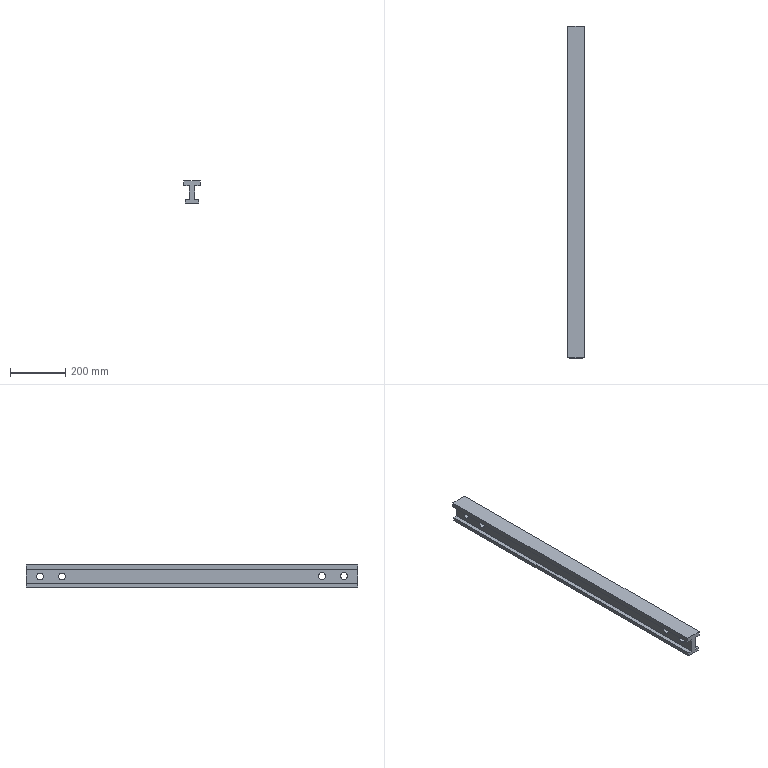Part | SolidWorks | features Extrusion 1, ICE 1 | 1 solid | 22 faces | box 60 x 1200 x 80 mm | volume 3164730 mm3 | plane 14 | cylinder 8 | commonest cylinder face diameters 25 x8
STEP:
#1=CARTESIAN_POINT('',(-10.,1150.,-14.417));
#2=VERTEX_POINT('',#1);
#3=CARTESIAN_POINT('',(-10.,1150.,10.583));
#4=VERTEX_POINT('',#3);
#5=CARTESIAN_POINT('',(-10.,1150.,-1.917));
#6=DIRECTION('',(-1.,0.,0.));
#7=DIRECTION('',(0.,0.,-1.));
#8=AXIS2_PLACEMENT_3D('',#5,#6,#7);
#9=CIRCLE('',#8,12.5);
#10=EDGE_CURVE('',#2,#4,#9,.T.);
#11=ORIENTED_EDGE('',*,*,#10,.T.);
#12=CARTESIAN_POINT('',(10.,1150.,10.583));
#13=VERTEX_POINT('',#12);
#14=CARTESIAN_POINT('',(-30.001,1150.,10.583));
#15=DIRECTION('',(1.,0.,0.));
#16=VECTOR('',#15,1000.);
#17=LINE('',#14,#16);
#18=EDGE_CURVE('',#4,#13,#17,.T.);
#19=ORIENTED_EDGE('',*,*,#18,.T.);
#20=CARTESIAN_POINT('',(10.,1150.,-14.417));
#21=VERTEX_POINT('',#20);
#22=CARTESIAN_POINT('',(10.,1150.,-1.917));
#23=DIRECTION('',(1.,0.,0.));
#24=DIRECTION('',(0.,0.,-1.));
#25=AXIS2_PLACEMENT_3D('',#22,#23,#24);
#26=CIRCLE('',#25,12.5);
#27=EDGE_CURVE('',#13,#21,#26,.T.);
#28=ORIENTED_EDGE('',*,*,#27,.T.);
#29=CARTESIAN_POINT('',(-30.001,1150.,-14.417));
#30=DIRECTION('',(1.,0.,0.));
#31=VECTOR('',#30,1000.);
#32=LINE('',#29,#31);
#33=EDGE_CURVE('',#2,#21,#32,.T.);
#34=ORIENTED_EDGE('',*,*,#33,.F.);
#35=EDGE_LOOP('',(#11,#19,#28,#34));
#36=FACE_OUTER_BOUND('',#35,.T.);
#37=CARTESIAN_POINT('',(-30.001,1150.,-1.917));
#38=DIRECTION('',(1.,0.,0.));
#39=DIRECTION('',(0.,0.,-1.));
#40=AXIS2_PLACEMENT_3D('',#37,#38,#39);
#41=CYLINDRICAL_SURFACE('',#40,12.5);
#42=ADVANCED_FACE('',(#36),#41,.F.);
#43=CARTESIAN_POINT('',(-10.,130.,-12.717));
#44=VERTEX_POINT('',#43);
#45=CARTESIAN_POINT('',(-10.,130.,12.283));
#46=VERTEX_POINT('',#45);
#47=CARTESIAN_POINT('',(-10.,130.,-0.2167));
#48=DIRECTION('',(-1.,0.,0.));
#49=DIRECTION('',(0.,0.,-1.));
#50=AXIS2_PLACEMENT_3D('',#47,#48,#49);
#51=CIRCLE('',#50,12.5);
#52=EDGE_CURVE('',#44,#46,#51,.T.);
#53=ORIENTED_EDGE('',*,*,#52,.T.);
#54=CARTESIAN_POINT('',(10.,130.,12.283));
#55=VERTEX_POINT('',#54);
#56=CARTESIAN_POINT('',(-30.001,130.,12.283));
#57=DIRECTION('',(1.,0.,0.));
#58=VECTOR('',#57,1000.);
#59=LINE('',#56,#58);
#60=EDGE_CURVE('',#46,#55,#59,.T.);
#61=ORIENTED_EDGE('',*,*,#60,.T.);
#62=CARTESIAN_POINT('',(10.,130.,-12.717));
#63=VERTEX_POINT('',#62);
#64=CARTESIAN_POINT('',(10.,130.,-0.2167));
#65=DIRECTION('',(1.,0.,0.));
#66=DIRECTION('',(0.,0.,-1.));
#67=AXIS2_PLACEMENT_3D('',#64,#65,#66);
#68=CIRCLE('',#67,12.5);
#69=EDGE_CURVE('',#55,#63,#68,.T.);
#70=ORIENTED_EDGE('',*,*,#69,.T.);
#71=CARTESIAN_POINT('',(-30.001,130.,-12.717));
#72=DIRECTION('',(1.,0.,0.));
#73=VECTOR('',#72,1000.);
#74=LINE('',#71,#73);
#75=EDGE_CURVE('',#44,#63,#74,.T.);
#76=ORIENTED_EDGE('',*,*,#75,.F.);
#77=EDGE_LOOP('',(#53,#61,#70,#76));
#78=FACE_OUTER_BOUND('',#77,.T.);
#79=CARTESIAN_POINT('',(-30.001,130.,-0.2167));
#80=DIRECTION('',(1.,0.,0.));
#81=DIRECTION('',(0.,0.,-1.));
#82=AXIS2_PLACEMENT_3D('',#79,#80,#81);
#83=CYLINDRICAL_SURFACE('',#82,12.5);
#84=ADVANCED_FACE('',(#78),#83,.F.);
#85=CARTESIAN_POINT('',(-10.,50.,-12.583));
#86=VERTEX_POINT('',#85);
#87=CARTESIAN_POINT('',(-10.,50.,12.417));
#88=VERTEX_POINT('',#87);
#89=CARTESIAN_POINT('',(-10.,50.,-0.08333));
#90=DIRECTION('',(-1.,0.,0.));
#91=DIRECTION('',(0.,0.,-1.));
#92=AXIS2_PLACEMENT_3D('',#89,#90,#91);
#93=CIRCLE('',#92,12.5);
#94=EDGE_CURVE('',#86,#88,#93,.T.);
#95=ORIENTED_EDGE('',*,*,#94,.T.);
#96=CARTESIAN_POINT('',(10.,50.,12.417));
#97=VERTEX_POINT('',#96);
#98=CARTESIAN_POINT('',(-30.001,50.,12.417));
#99=DIRECTION('',(1.,0.,0.));
#100=VECTOR('',#99,1000.);
#101=LINE('',#98,#100);
#102=EDGE_CURVE('',#88,#97,#101,.T.);
#103=ORIENTED_EDGE('',*,*,#102,.T.);
#104=CARTESIAN_POINT('',(10.,50.,-12.583));
#105=VERTEX_POINT('',#104);
#106=CARTESIAN_POINT('',(10.,50.,-0.08333));
#107=DIRECTION('',(1.,0.,0.));
#108=DIRECTION('',(0.,0.,-1.));
#109=AXIS2_PLACEMENT_3D('',#106,#107,#108);
#110=CIRCLE('',#109,12.5);
#111=EDGE_CURVE('',#97,#105,#110,.T.);
#112=ORIENTED_EDGE('',*,*,#111,.T.);
#113=CARTESIAN_POINT('',(-30.001,50.,-12.583));
#114=DIRECTION('',(1.,0.,0.));
#115=VECTOR('',#114,1000.);
#116=LINE('',#113,#115);
#117=EDGE_CURVE('',#86,#105,#116,.T.);
#118=ORIENTED_EDGE('',*,*,#117,.F.);
#119=EDGE_LOOP('',(#95,#103,#112,#118));
#120=FACE_OUTER_BOUND('',#119,.T.);
#121=CARTESIAN_POINT('',(-30.001,50.,-0.08333));
#122=DIRECTION('',(1.,0.,0.));
#123=DIRECTION('',(0.,0.,-1.));
#124=AXIS2_PLACEMENT_3D('',#121,#122,#123);
#125=CYLINDRICAL_SURFACE('',#124,12.5);
#126=ADVANCED_FACE('',(#120),#125,.F.);
#127=CARTESIAN_POINT('',(-10.,1070.,-14.283));
#128=VERTEX_POINT('',#127);
#129=CARTESIAN_POINT('',(-10.,1070.,10.717));
#130=VERTEX_POINT('',#129);
#131=CARTESIAN_POINT('',(-10.,1070.,-1.783));
#132=DIRECTION('',(-1.,0.,0.));
#133=DIRECTION('',(0.,0.,-1.));
#134=AXIS2_PLACEMENT_3D('',#131,#132,#133);
#135=CIRCLE('',#134,12.5);
#136=EDGE_CURVE('',#128,#130,#135,.T.);
#137=ORIENTED_EDGE('',*,*,#136,.T.);
#138=CARTESIAN_POINT('',(10.,1070.,10.717));
#139=VERTEX_POINT('',#138);
#140=CARTESIAN_POINT('',(-30.001,1070.,10.717));
#141=DIRECTION('',(1.,0.,0.));
#142=VECTOR('',#141,1000.);
#143=LINE('',#140,#142);
#144=EDGE_CURVE('',#130,#139,#143,.T.);
#145=ORIENTED_EDGE('',*,*,#144,.T.);
#146=CARTESIAN_POINT('',(10.,1070.,-14.283));
#147=VERTEX_POINT('',#146);
#148=CARTESIAN_POINT('',(10.,1070.,-1.783));
#149=DIRECTION('',(1.,0.,0.));
#150=DIRECTION('',(0.,0.,-1.));
#151=AXIS2_PLACEMENT_3D('',#148,#149,#150);
#152=CIRCLE('',#151,12.5);
#153=EDGE_CURVE('',#139,#147,#152,.T.);
#154=ORIENTED_EDGE('',*,*,#153,.T.);
#155=CARTESIAN_POINT('',(-30.001,1070.,-14.283));
#156=DIRECTION('',(1.,0.,0.));
#157=VECTOR('',#156,1000.);
#158=LINE('',#155,#157);
#159=EDGE_CURVE('',#128,#147,#158,.T.);
#160=ORIENTED_EDGE('',*,*,#159,.F.);
#161=EDGE_LOOP('',(#137,#145,#154,#160));
#162=FACE_OUTER_BOUND('',#161,.T.);
#163=CARTESIAN_POINT('',(-30.001,1070.,-1.783));
#164=DIRECTION('',(1.,0.,0.));
#165=DIRECTION('',(0.,0.,-1.));
#166=AXIS2_PLACEMENT_3D('',#163,#164,#165);
#167=CYLINDRICAL_SURFACE('',#166,12.5);
#168=ADVANCED_FACE('',(#162),#167,.F.);
#169=CARTESIAN_POINT('',(-25.,0.,-40.));
#170=VERTEX_POINT('',#169);
#171=CARTESIAN_POINT('',(-25.,0.,-27.));
#172=VERTEX_POINT('',#171);
#173=CARTESIAN_POINT('',(-25.,0.,-40.));
#174=DIRECTION('',(0.,0.,1.));
#175=VECTOR('',#174,1000.);
#176=LINE('',#173,#175);
#177=EDGE_CURVE('',#170,#172,#176,.T.);
#178=ORIENTED_EDGE('',*,*,#177,.T.);
#179=CARTESIAN_POINT('',(-25.,1200.,-27.));
#180=VERTEX_POINT('',#179);
#181=CARTESIAN_POINT('',(-25.,1200.,-27.));
#182=DIRECTION('',(0.,-1.,0.));
#183=VECTOR('',#182,1000.);
#184=LINE('',#181,#183);
#185=EDGE_CURVE('',#180,#172,#184,.T.);
#186=ORIENTED_EDGE('',*,*,#185,.F.);
#187=CARTESIAN_POINT('',(-25.,1200.,-40.));
#188=VERTEX_POINT('',#187);
#189=CARTESIAN_POINT('',(-25.,1200.,-40.));
#190=DIRECTION('',(0.,0.,1.));
#191=VECTOR('',#190,1000.);
#192=LINE('',#189,#191);
#193=EDGE_CURVE('',#188,#180,#192,.T.);
#194=ORIENTED_EDGE('',*,*,#193,.F.);
#195=CARTESIAN_POINT('',(-25.,1200.,-40.));
#196=DIRECTION('',(0.,-1.,0.));
#197=VECTOR('',#196,1000.);
#198=LINE('',#195,#197);
#199=EDGE_CURVE('',#188,#170,#198,.T.);
#200=ORIENTED_EDGE('',*,*,#199,.T.);
#201=EDGE_LOOP('',(#178,#186,#194,#200));
#202=FACE_OUTER_BOUND('',#201,.T.);
#203=CARTESIAN_POINT('',(-25.,1200.,-40.));
#204=DIRECTION('',(1.,0.,0.));
#205=DIRECTION('',(0.,0.,-1.));
#206=AXIS2_PLACEMENT_3D('',#203,#204,#205);
#207=PLANE('',#206);
#208=ADVANCED_FACE('',(#202),#207,.F.);
#209=CARTESIAN_POINT('',(-10.,0.,-27.));
#210=VERTEX_POINT('',#209);
#211=CARTESIAN_POINT('',(-25.,0.,-27.));
#212=DIRECTION('',(1.,0.,0.));
#213=VECTOR('',#212,1000.);
#214=LINE('',#211,#213);
#215=EDGE_CURVE('',#172,#210,#214,.T.);
#216=ORIENTED_EDGE('',*,*,#215,.T.);
#217=CARTESIAN_POINT('',(-10.,1200.,-27.));
#218=VERTEX_POINT('',#217);
#219=CARTESIAN_POINT('',(-10.,1200.,-27.));
#220=DIRECTION('',(0.,-1.,0.));
#221=VECTOR('',#220,1000.);
#222=LINE('',#219,#221);
#223=EDGE_CURVE('',#218,#210,#222,.T.);
#224=ORIENTED_EDGE('',*,*,#223,.F.);
#225=CARTESIAN_POINT('',(-25.,1200.,-27.));
#226=DIRECTION('',(1.,0.,0.));
#227=VECTOR('',#226,1000.);
#228=LINE('',#225,#227);
#229=EDGE_CURVE('',#180,#218,#228,.T.);
#230=ORIENTED_EDGE('',*,*,#229,.F.);
#231=ORIENTED_EDGE('',*,*,#185,.T.);
#232=EDGE_LOOP('',(#216,#224,#230,#231));
#233=FACE_OUTER_BOUND('',#232,.T.);
#234=CARTESIAN_POINT('',(-25.,1200.,-27.));
#235=DIRECTION('',(0.,0.,-1.));
#236=DIRECTION('',(-1.,0.,0.));
#237=AXIS2_PLACEMENT_3D('',#234,#235,#236);
#238=PLANE('',#237);
#239=ADVANCED_FACE('',(#233),#238,.F.);
#240=ORIENTED_EDGE('',*,*,#10,.F.);
#241=CARTESIAN_POINT('',(-10.,1150.,-1.917));
#242=DIRECTION('',(-1.,0.,0.));
#243=DIRECTION('',(0.,0.,-1.));
#244=AXIS2_PLACEMENT_3D('',#241,#242,#243);
#245=CIRCLE('',#244,12.5);
#246=EDGE_CURVE('',#4,#2,#245,.T.);
#247=ORIENTED_EDGE('',*,*,#246,.F.);
#248=EDGE_LOOP('',(#240,#247));
#249=FACE_BOUND('',#248,.T.);
#250=ORIENTED_EDGE('',*,*,#52,.F.);
#251=CARTESIAN_POINT('',(-10.,130.,-0.2167));
#252=DIRECTION('',(-1.,0.,0.));
#253=DIRECTION('',(0.,0.,-1.));
#254=AXIS2_PLACEMENT_3D('',#251,#252,#253);
#255=CIRCLE('',#254,12.5);
#256=EDGE_CURVE('',#46,#44,#255,.T.);
#257=ORIENTED_EDGE('',*,*,#256,.F.);
#258=EDGE_LOOP('',(#250,#257));
#259=FACE_BOUND('',#258,.T.);
#260=ORIENTED_EDGE('',*,*,#94,.F.);
#261=CARTESIAN_POINT('',(-10.,50.,-0.08333));
#262=DIRECTION('',(-1.,0.,0.));
#263=DIRECTION('',(0.,0.,-1.));
#264=AXIS2_PLACEMENT_3D('',#261,#262,#263);
#265=CIRCLE('',#264,12.5);
#266=EDGE_CURVE('',#88,#86,#265,.T.);
#267=ORIENTED_EDGE('',*,*,#266,.F.);
#268=EDGE_LOOP('',(#260,#267));
#269=FACE_BOUND('',#268,.T.);
#270=ORIENTED_EDGE('',*,*,#136,.F.);
#271=CARTESIAN_POINT('',(-10.,1070.,-1.783));
#272=DIRECTION('',(-1.,0.,0.));
#273=DIRECTION('',(0.,0.,-1.));
#274=AXIS2_PLACEMENT_3D('',#271,#272,#273);
#275=CIRCLE('',#274,12.5);
#276=EDGE_CURVE('',#130,#128,#275,.T.);
#277=ORIENTED_EDGE('',*,*,#276,.F.);
#278=EDGE_LOOP('',(#270,#277));
#279=FACE_BOUND('',#278,.T.);
#280=CARTESIAN_POINT('',(-10.,0.,23.));
#281=VERTEX_POINT('',#280);
#282=CARTESIAN_POINT('',(-10.,0.,-27.));
#283=DIRECTION('',(0.,0.,1.));
#284=VECTOR('',#283,1000.);
#285=LINE('',#282,#284);
#286=EDGE_CURVE('',#210,#281,#285,.T.);
#287=ORIENTED_EDGE('',*,*,#286,.T.);
#288=CARTESIAN_POINT('',(-10.,1200.,23.));
#289=VERTEX_POINT('',#288);
#290=CARTESIAN_POINT('',(-10.,1200.,23.));
#291=DIRECTION('',(0.,-1.,0.));
#292=VECTOR('',#291,1000.);
#293=LINE('',#290,#292);
#294=EDGE_CURVE('',#289,#281,#293,.T.);
#295=ORIENTED_EDGE('',*,*,#294,.F.);
#296=CARTESIAN_POINT('',(-10.,1200.,-27.));
#297=DIRECTION('',(0.,0.,1.));
#298=VECTOR('',#297,1000.);
#299=LINE('',#296,#298);
#300=EDGE_CURVE('',#218,#289,#299,.T.);
#301=ORIENTED_EDGE('',*,*,#300,.F.);
#302=ORIENTED_EDGE('',*,*,#223,.T.);
#303=EDGE_LOOP('',(#287,#295,#301,#302));
#304=FACE_OUTER_BOUND('',#303,.T.);
#305=CARTESIAN_POINT('',(-10.,1200.,-27.));
#306=DIRECTION('',(1.,0.,0.));
#307=DIRECTION('',(0.,0.,-1.));
#308=AXIS2_PLACEMENT_3D('',#305,#306,#307);
#309=PLANE('',#308);
#310=ADVANCED_FACE('',(#249,#259,#269,#279,#304),#309,.F.);
#311=CARTESIAN_POINT('',(-30.,0.,23.));
#312=VERTEX_POINT('',#311);
#313=CARTESIAN_POINT('',(-10.,0.,23.));
#314=DIRECTION('',(-1.,0.,0.));
#315=VECTOR('',#314,1000.);
#316=LINE('',#313,#315);
#317=EDGE_CURVE('',#281,#312,#316,.T.);
#318=ORIENTED_EDGE('',*,*,#317,.T.);
#319=CARTESIAN_POINT('',(-30.,1200.,23.));
#320=VERTEX_POINT('',#319);
#321=CARTESIAN_POINT('',(-30.,1200.,23.));
#322=DIRECTION('',(0.,-1.,0.));
#323=VECTOR('',#322,1000.);
#324=LINE('',#321,#323);
#325=EDGE_CURVE('',#320,#312,#324,.T.);
#326=ORIENTED_EDGE('',*,*,#325,.F.);
#327=CARTESIAN_POINT('',(-10.,1200.,23.));
#328=DIRECTION('',(-1.,0.,0.));
#329=VECTOR('',#328,1000.);
#330=LINE('',#327,#329);
#331=EDGE_CURVE('',#289,#320,#330,.T.);
#332=ORIENTED_EDGE('',*,*,#331,.F.);
#333=ORIENTED_EDGE('',*,*,#294,.T.);
#334=EDGE_LOOP('',(#318,#326,#332,#333));
#335=FACE_OUTER_BOUND('',#334,.T.);
#336=CARTESIAN_POINT('',(-10.,1200.,23.));
#337=DIRECTION('',(0.,0.,1.));
#338=DIRECTION('',(1.,0.,0.));
#339=AXIS2_PLACEMENT_3D('',#336,#337,#338);
#340=PLANE('',#339);
#341=ADVANCED_FACE('',(#335),#340,.F.);
#342=CARTESIAN_POINT('',(-30.,0.,40.));
#343=VERTEX_POINT('',#342);
#344=CARTESIAN_POINT('',(-30.,0.,40.));
#345=DIRECTION('',(0.,0.,1.));
#346=VECTOR('',#345,1000.);
#347=LINE('',#344,#346);
#348=EDGE_CURVE('',#312,#343,#347,.T.);
#349=ORIENTED_EDGE('',*,*,#348,.T.);
#350=CARTESIAN_POINT('',(-30.,1200.,40.));
#351=VERTEX_POINT('',#350);
#352=CARTESIAN_POINT('',(-30.,1200.,40.));
#353=DIRECTION('',(0.,-1.,0.));
#354=VECTOR('',#353,1000.);
#355=LINE('',#352,#354);
#356=EDGE_CURVE('',#351,#343,#355,.T.);
#357=ORIENTED_EDGE('',*,*,#356,.F.);
#358=CARTESIAN_POINT('',(-30.,1200.,40.));
#359=DIRECTION('',(0.,0.,1.));
#360=VECTOR('',#359,1000.);
#361=LINE('',#358,#360);
#362=EDGE_CURVE('',#320,#351,#361,.T.);
#363=ORIENTED_EDGE('',*,*,#362,.F.);
#364=ORIENTED_EDGE('',*,*,#325,.T.);
#365=EDGE_LOOP('',(#349,#357,#363,#364));
#366=FACE_OUTER_BOUND('',#365,.T.);
#367=CARTESIAN_POINT('',(-30.,1200.,40.));
#368=DIRECTION('',(1.,0.,0.));
#369=DIRECTION('',(0.,0.,-1.));
#370=AXIS2_PLACEMENT_3D('',#367,#368,#369);
#371=PLANE('',#370);
#372=ADVANCED_FACE('',(#366),#371,.F.);
#373=CARTESIAN_POINT('',(30.,0.,40.));
#374=VERTEX_POINT('',#373);
#375=CARTESIAN_POINT('',(30.,0.,40.));
#376=DIRECTION('',(1.,0.,0.));
#377=VECTOR('',#376,1000.);
#378=LINE('',#375,#377);
#379=EDGE_CURVE('',#343,#374,#378,.T.);
#380=ORIENTED_EDGE('',*,*,#379,.T.);
#381=CARTESIAN_POINT('',(30.,1200.,40.));
#382=VERTEX_POINT('',#381);
#383=CARTESIAN_POINT('',(30.,1200.,40.));
#384=DIRECTION('',(0.,-1.,0.));
#385=VECTOR('',#384,1000.);
#386=LINE('',#383,#385);
#387=EDGE_CURVE('',#382,#374,#386,.T.);
#388=ORIENTED_EDGE('',*,*,#387,.F.);
#389=CARTESIAN_POINT('',(30.,1200.,40.));
#390=DIRECTION('',(1.,0.,0.));
#391=VECTOR('',#390,1000.);
#392=LINE('',#389,#391);
#393=EDGE_CURVE('',#351,#382,#392,.T.);
#394=ORIENTED_EDGE('',*,*,#393,.F.);
#395=ORIENTED_EDGE('',*,*,#356,.T.);
#396=EDGE_LOOP('',(#380,#388,#394,#395));
#397=FACE_OUTER_BOUND('',#396,.T.);
#398=CARTESIAN_POINT('',(30.,1200.,40.));
#399=DIRECTION('',(0.,0.,-1.));
#400=DIRECTION('',(-1.,0.,0.));
#401=AXIS2_PLACEMENT_3D('',#398,#399,#400);
#402=PLANE('',#401);
#403=ADVANCED_FACE('',(#397),#402,.F.);
#404=CARTESIAN_POINT('',(30.,0.,23.));
#405=VERTEX_POINT('',#404);
#406=CARTESIAN_POINT('',(30.,0.,40.));
#407=DIRECTION('',(0.,0.,-1.));
#408=VECTOR('',#407,1000.);
#409=LINE('',#406,#408);
#410=EDGE_CURVE('',#374,#405,#409,.T.);
#411=ORIENTED_EDGE('',*,*,#410,.T.);
#412=CARTESIAN_POINT('',(30.,1200.,23.));
#413=VERTEX_POINT('',#412);
#414=CARTESIAN_POINT('',(30.,1200.,23.));
#415=DIRECTION('',(0.,-1.,0.));
#416=VECTOR('',#415,1000.);
#417=LINE('',#414,#416);
#418=EDGE_CURVE('',#413,#405,#417,.T.);
#419=ORIENTED_EDGE('',*,*,#418,.F.);
#420=CARTESIAN_POINT('',(30.,1200.,40.));
#421=DIRECTION('',(0.,0.,-1.));
#422=VECTOR('',#421,1000.);
#423=LINE('',#420,#422);
#424=EDGE_CURVE('',#382,#413,#423,.T.);
#425=ORIENTED_EDGE('',*,*,#424,.F.);
#426=ORIENTED_EDGE('',*,*,#387,.T.);
#427=EDGE_LOOP('',(#411,#419,#425,#426));
#428=FACE_OUTER_BOUND('',#427,.T.);
#429=CARTESIAN_POINT('',(30.,1200.,40.));
#430=DIRECTION('',(-1.,0.,0.));
#431=DIRECTION('',(0.,0.,1.));
#432=AXIS2_PLACEMENT_3D('',#429,#430,#431);
#433=PLANE('',#432);
#434=ADVANCED_FACE('',(#428),#433,.F.);
#435=CARTESIAN_POINT('',(10.,0.,23.));
#436=VERTEX_POINT('',#435);
#437=CARTESIAN_POINT('',(30.,0.,23.));
#438=DIRECTION('',(-1.,0.,0.));
#439=VECTOR('',#438,1000.);
#440=LINE('',#437,#439);
#441=EDGE_CURVE('',#405,#436,#440,.T.);
#442=ORIENTED_EDGE('',*,*,#441,.T.);
#443=CARTESIAN_POINT('',(10.,1200.,23.));
#444=VERTEX_POINT('',#443);
#445=CARTESIAN_POINT('',(10.,1200.,23.));
#446=DIRECTION('',(0.,-1.,0.));
#447=VECTOR('',#446,1000.);
#448=LINE('',#445,#447);
#449=EDGE_CURVE('',#444,#436,#448,.T.);
#450=ORIENTED_EDGE('',*,*,#449,.F.);
#451=CARTESIAN_POINT('',(30.,1200.,23.));
#452=DIRECTION('',(-1.,0.,0.));
#453=VECTOR('',#452,1000.);
#454=LINE('',#451,#453);
#455=EDGE_CURVE('',#413,#444,#454,.T.);
#456=ORIENTED_EDGE('',*,*,#455,.F.);
#457=ORIENTED_EDGE('',*,*,#418,.T.);
#458=EDGE_LOOP('',(#442,#450,#456,#457));
#459=FACE_OUTER_BOUND('',#458,.T.);
#460=CARTESIAN_POINT('',(30.,1200.,23.));
#461=DIRECTION('',(0.,0.,1.));
#462=DIRECTION('',(1.,0.,0.));
#463=AXIS2_PLACEMENT_3D('',#460,#461,#462);
#464=PLANE('',#463);
#465=ADVANCED_FACE('',(#459),#464,.F.);
#466=CARTESIAN_POINT('',(10.,1150.,-1.917));
#467=DIRECTION('',(1.,0.,0.));
#468=DIRECTION('',(0.,0.,-1.));
#469=AXIS2_PLACEMENT_3D('',#466,#467,#468);
#470=CIRCLE('',#469,12.5);
#471=EDGE_CURVE('',#21,#13,#470,.T.);
#472=ORIENTED_EDGE('',*,*,#471,.F.);
#473=ORIENTED_EDGE('',*,*,#27,.F.);
#474=EDGE_LOOP('',(#472,#473));
#475=FACE_BOUND('',#474,.T.);
#476=CARTESIAN_POINT('',(10.,130.,-0.2167));
#477=DIRECTION('',(1.,0.,0.));
#478=DIRECTION('',(0.,0.,-1.));
#479=AXIS2_PLACEMENT_3D('',#476,#477,#478);
#480=CIRCLE('',#479,12.5);
#481=EDGE_CURVE('',#63,#55,#480,.T.);
#482=ORIENTED_EDGE('',*,*,#481,.F.);
#483=ORIENTED_EDGE('',*,*,#69,.F.);
#484=EDGE_LOOP('',(#482,#483));
#485=FACE_BOUND('',#484,.T.);
#486=CARTESIAN_POINT('',(10.,50.,-0.08333));
#487=DIRECTION('',(1.,0.,0.));
#488=DIRECTION('',(0.,0.,-1.));
#489=AXIS2_PLACEMENT_3D('',#486,#487,#488);
#490=CIRCLE('',#489,12.5);
#491=EDGE_CURVE('',#105,#97,#490,.T.);
#492=ORIENTED_EDGE('',*,*,#491,.F.);
#493=ORIENTED_EDGE('',*,*,#111,.F.);
#494=EDGE_LOOP('',(#492,#493));
#495=FACE_BOUND('',#494,.T.);
#496=CARTESIAN_POINT('',(10.,1070.,-1.783));
#497=DIRECTION('',(1.,0.,0.));
#498=DIRECTION('',(0.,0.,-1.));
#499=AXIS2_PLACEMENT_3D('',#496,#497,#498);
#500=CIRCLE('',#499,12.5);
#501=EDGE_CURVE('',#147,#139,#500,.T.);
#502=ORIENTED_EDGE('',*,*,#501,.F.);
#503=ORIENTED_EDGE('',*,*,#153,.F.);
#504=EDGE_LOOP('',(#502,#503));
#505=FACE_BOUND('',#504,.T.);
#506=CARTESIAN_POINT('',(10.,0.,-27.));
#507=VERTEX_POINT('',#506);
#508=CARTESIAN_POINT('',(10.,0.,-27.));
#509=DIRECTION('',(0.,0.,-1.));
#510=VECTOR('',#509,1000.);
#511=LINE('',#508,#510);
#512=EDGE_CURVE('',#436,#507,#511,.T.);
#513=ORIENTED_EDGE('',*,*,#512,.T.);
#514=CARTESIAN_POINT('',(10.,1200.,-27.));
#515=VERTEX_POINT('',#514);
#516=CARTESIAN_POINT('',(10.,1200.,-27.));
#517=DIRECTION('',(0.,-1.,0.));
#518=VECTOR('',#517,1000.);
#519=LINE('',#516,#518);
#520=EDGE_CURVE('',#515,#507,#519,.T.);
#521=ORIENTED_EDGE('',*,*,#520,.F.);
#522=CARTESIAN_POINT('',(10.,1200.,-27.));
#523=DIRECTION('',(0.,0.,-1.));
#524=VECTOR('',#523,1000.);
#525=LINE('',#522,#524);
#526=EDGE_CURVE('',#444,#515,#525,.T.);
#527=ORIENTED_EDGE('',*,*,#526,.F.);
#528=ORIENTED_EDGE('',*,*,#449,.T.);
#529=EDGE_LOOP('',(#513,#521,#527,#528));
#530=FACE_OUTER_BOUND('',#529,.T.);
#531=CARTESIAN_POINT('',(10.,1200.,-27.));
#532=DIRECTION('',(-1.,0.,0.));
#533=DIRECTION('',(0.,0.,1.));
#534=AXIS2_PLACEMENT_3D('',#531,#532,#533);
#535=PLANE('',#534);
#536=ADVANCED_FACE('',(#475,#485,#495,#505,#530),#535,.F.);
#537=CARTESIAN_POINT('',(25.,0.,-27.));
#538=VERTEX_POINT('',#537);
#539=CARTESIAN_POINT('',(10.,0.,-27.));
#540=DIRECTION('',(1.,0.,0.));
#541=VECTOR('',#540,1000.);
#542=LINE('',#539,#541);
#543=EDGE_CURVE('',#507,#538,#542,.T.);
#544=ORIENTED_EDGE('',*,*,#543,.T.);
#545=CARTESIAN_POINT('',(25.,1200.,-27.));
#546=VERTEX_POINT('',#545);
#547=CARTESIAN_POINT('',(25.,1200.,-27.));
#548=DIRECTION('',(0.,-1.,0.));
#549=VECTOR('',#548,1000.);
#550=LINE('',#547,#549);
#551=EDGE_CURVE('',#546,#538,#550,.T.);
#552=ORIENTED_EDGE('',*,*,#551,.F.);
#553=CARTESIAN_POINT('',(10.,1200.,-27.));
#554=DIRECTION('',(1.,0.,0.));
#555=VECTOR('',#554,1000.);
#556=LINE('',#553,#555);
#557=EDGE_CURVE('',#515,#546,#556,.T.);
#558=ORIENTED_EDGE('',*,*,#557,.F.);
#559=ORIENTED_EDGE('',*,*,#520,.T.);
#560=EDGE_LOOP('',(#544,#552,#558,#559));
#561=FACE_OUTER_BOUND('',#560,.T.);
#562=CARTESIAN_POINT('',(10.,1200.,-27.));
#563=DIRECTION('',(0.,0.,-1.));
#564=DIRECTION('',(-1.,0.,0.));
#565=AXIS2_PLACEMENT_3D('',#562,#563,#564);
#566=PLANE('',#565);
#567=ADVANCED_FACE('',(#561),#566,.F.);
#568=CARTESIAN_POINT('',(25.,0.,-40.));
#569=VERTEX_POINT('',#568);
#570=CARTESIAN_POINT('',(25.,0.,-40.));
#571=DIRECTION('',(0.,0.,-1.));
#572=VECTOR('',#571,1000.);
#573=LINE('',#570,#572);
#574=EDGE_CURVE('',#538,#569,#573,.T.);
#575=ORIENTED_EDGE('',*,*,#574,.T.);
#576=CARTESIAN_POINT('',(25.,1200.,-40.));
#577=VERTEX_POINT('',#576);
#578=CARTESIAN_POINT('',(25.,1200.,-40.));
#579=DIRECTION('',(0.,-1.,0.));
#580=VECTOR('',#579,1000.);
#581=LINE('',#578,#580);
#582=EDGE_CURVE('',#577,#569,#581,.T.);
#583=ORIENTED_EDGE('',*,*,#582,.F.);
#584=CARTESIAN_POINT('',(25.,1200.,-40.));
#585=DIRECTION('',(0.,0.,-1.));
#586=VECTOR('',#585,1000.);
#587=LINE('',#584,#586);
#588=EDGE_CURVE('',#546,#577,#587,.T.);
#589=ORIENTED_EDGE('',*,*,#588,.F.);
#590=ORIENTED_EDGE('',*,*,#551,.T.);
#591=EDGE_LOOP('',(#575,#583,#589,#590));
#592=FACE_OUTER_BOUND('',#591,.T.);
#593=CARTESIAN_POINT('',(25.,1200.,-40.));
#594=DIRECTION('',(-1.,0.,0.));
#595=DIRECTION('',(0.,0.,1.));
#596=AXIS2_PLACEMENT_3D('',#593,#594,#595);
#597=PLANE('',#596);
#598=ADVANCED_FACE('',(#592),#597,.F.);
#599=CARTESIAN_POINT('',(-25.,0.,-40.));
#600=DIRECTION('',(-1.,0.,0.));
#601=VECTOR('',#600,1000.);
#602=LINE('',#599,#601);
#603=EDGE_CURVE('',#569,#170,#602,.T.);
#604=ORIENTED_EDGE('',*,*,#603,.T.);
#605=ORIENTED_EDGE('',*,*,#199,.F.);
#606=CARTESIAN_POINT('',(-25.,1200.,-40.));
#607=DIRECTION('',(-1.,0.,0.));
#608=VECTOR('',#607,1000.);
#609=LINE('',#606,#608);
#610=EDGE_CURVE('',#577,#188,#609,.T.);
#611=ORIENTED_EDGE('',*,*,#610,.F.);
#612=ORIENTED_EDGE('',*,*,#582,.T.);
#613=EDGE_LOOP('',(#604,#605,#611,#612));
#614=FACE_OUTER_BOUND('',#613,.T.);
#615=CARTESIAN_POINT('',(-25.,1200.,-40.));
#616=DIRECTION('',(0.,0.,1.));
#617=DIRECTION('',(1.,0.,0.));
#618=AXIS2_PLACEMENT_3D('',#615,#616,#617);
#619=PLANE('',#618);
#620=ADVANCED_FACE('',(#614),#619,.F.);
#621=ORIENTED_EDGE('',*,*,#193,.T.);
#622=ORIENTED_EDGE('',*,*,#229,.T.);
#623=ORIENTED_EDGE('',*,*,#300,.T.);
#624=ORIENTED_EDGE('',*,*,#331,.T.);
#625=ORIENTED_EDGE('',*,*,#362,.T.);
#626=ORIENTED_EDGE('',*,*,#393,.T.);
#627=ORIENTED_EDGE('',*,*,#424,.T.);
#628=ORIENTED_EDGE('',*,*,#455,.T.);
#629=ORIENTED_EDGE('',*,*,#526,.T.);
#630=ORIENTED_EDGE('',*,*,#557,.T.);
#631=ORIENTED_EDGE('',*,*,#588,.T.);
#632=ORIENTED_EDGE('',*,*,#610,.T.);
#633=EDGE_LOOP('',(#621,#622,#623,#624,#625,#626,#627,#628,#629,#630,#631,#632));
#634=FACE_OUTER_BOUND('',#633,.T.);
#635=CARTESIAN_POINT('',(0.,1200.,0.));
#636=DIRECTION('',(0.,1.,0.));
#637=DIRECTION('',(0.,0.,1.));
#638=AXIS2_PLACEMENT_3D('',#635,#636,#637);
#639=PLANE('',#638);
#640=ADVANCED_FACE('',(#634),#639,.T.);
#641=ORIENTED_EDGE('',*,*,#177,.F.);
#642=ORIENTED_EDGE('',*,*,#603,.F.);
#643=ORIENTED_EDGE('',*,*,#574,.F.);
#644=ORIENTED_EDGE('',*,*,#543,.F.);
#645=ORIENTED_EDGE('',*,*,#512,.F.);
#646=ORIENTED_EDGE('',*,*,#441,.F.);
#647=ORIENTED_EDGE('',*,*,#410,.F.);
#648=ORIENTED_EDGE('',*,*,#379,.F.);
#649=ORIENTED_EDGE('',*,*,#348,.F.);
#650=ORIENTED_EDGE('',*,*,#317,.F.);
#651=ORIENTED_EDGE('',*,*,#286,.F.);
#652=ORIENTED_EDGE('',*,*,#215,.F.);
#653=EDGE_LOOP('',(#641,#642,#643,#644,#645,#646,#647,#648,#649,#650,#651,#652));
#654=FACE_OUTER_BOUND('',#653,.T.);
#655=CARTESIAN_POINT('',(0.,0.,0.));
#656=DIRECTION('',(0.,1.,0.));
#657=DIRECTION('',(0.,0.,1.));
#658=AXIS2_PLACEMENT_3D('',#655,#656,#657);
#659=PLANE('',#658);
#660=ADVANCED_FACE('',(#654),#659,.F.);
#661=ORIENTED_EDGE('',*,*,#144,.F.);
#662=ORIENTED_EDGE('',*,*,#276,.T.);
#663=ORIENTED_EDGE('',*,*,#159,.T.);
#664=ORIENTED_EDGE('',*,*,#501,.T.);
#665=EDGE_LOOP('',(#661,#662,#663,#664));
#666=FACE_OUTER_BOUND('',#665,.T.);
#667=CARTESIAN_POINT('',(-30.001,1070.,-1.783));
#668=DIRECTION('',(1.,0.,0.));
#669=DIRECTION('',(0.,0.,-1.));
#670=AXIS2_PLACEMENT_3D('',#667,#668,#669);
#671=CYLINDRICAL_SURFACE('',#670,12.5);
#672=ADVANCED_FACE('',(#666),#671,.F.);
#673=ORIENTED_EDGE('',*,*,#102,.F.);
#674=ORIENTED_EDGE('',*,*,#266,.T.);
#675=ORIENTED_EDGE('',*,*,#117,.T.);
#676=ORIENTED_EDGE('',*,*,#491,.T.);
#677=EDGE_LOOP('',(#673,#674,#675,#676));
#678=FACE_OUTER_BOUND('',#677,.T.);
#679=CARTESIAN_POINT('',(-30.001,50.,-0.08333));
#680=DIRECTION('',(1.,0.,0.));
#681=DIRECTION('',(0.,0.,-1.));
#682=AXIS2_PLACEMENT_3D('',#679,#680,#681);
#683=CYLINDRICAL_SURFACE('',#682,12.5);
#684=ADVANCED_FACE('',(#678),#683,.F.);
#685=ORIENTED_EDGE('',*,*,#60,.F.);
#686=ORIENTED_EDGE('',*,*,#256,.T.);
#687=ORIENTED_EDGE('',*,*,#75,.T.);
#688=ORIENTED_EDGE('',*,*,#481,.T.);
#689=EDGE_LOOP('',(#685,#686,#687,#688));
#690=FACE_OUTER_BOUND('',#689,.T.);
#691=CARTESIAN_POINT('',(-30.001,130.,-0.2167));
#692=DIRECTION('',(1.,0.,0.));
#693=DIRECTION('',(0.,0.,-1.));
#694=AXIS2_PLACEMENT_3D('',#691,#692,#693);
#695=CYLINDRICAL_SURFACE('',#694,12.5);
#696=ADVANCED_FACE('',(#690),#695,.F.);
#697=ORIENTED_EDGE('',*,*,#18,.F.);
#698=ORIENTED_EDGE('',*,*,#246,.T.);
#699=ORIENTED_EDGE('',*,*,#33,.T.);
#700=ORIENTED_EDGE('',*,*,#471,.T.);
#701=EDGE_LOOP('',(#697,#698,#699,#700));
#702=FACE_OUTER_BOUND('',#701,.T.);
#703=CARTESIAN_POINT('',(-30.001,1150.,-1.917));
#704=DIRECTION('',(1.,0.,0.));
#705=DIRECTION('',(0.,0.,-1.));
#706=AXIS2_PLACEMENT_3D('',#703,#704,#705);
#707=CYLINDRICAL_SURFACE('',#706,12.5);
#708=ADVANCED_FACE('',(#702),#707,.F.);
#709=CLOSED_SHELL('',(#42,#84,#126,#168,#208,#239,#310,#341,#372,#403,#434,#465,#536,#567,#598,#620,#640,#660,#672,#684,#696,#708));
#710=MANIFOLD_SOLID_BREP('',#709);
#711=CARTESIAN_POINT('',(0.,0.,0.));
#712=DIRECTION('',(0.,0.,1.));
#713=DIRECTION('',(1.,0.,0.));
#714=AXIS2_PLACEMENT_3D('',#711,#712,#713);
#715=(LENGTH_UNIT()NAMED_UNIT(*)SI_UNIT(.MILLI.,.METRE.));
#716=UNCERTAINTY_MEASURE_WITH_UNIT(LENGTH_MEASURE(0.00001),#715,'','');
#717=(NAMED_UNIT(*)PLANE_ANGLE_UNIT()SI_UNIT($,.RADIAN.));
#718=(NAMED_UNIT(*)SI_UNIT($,.STERADIAN.)SOLID_ANGLE_UNIT());
#719=(GEOMETRIC_REPRESENTATION_CONTEXT(3)GLOBAL_UNCERTAINTY_ASSIGNED_CONTEXT((#716))GLOBAL_UNIT_ASSIGNED_CONTEXT((#715,#717,#718))REPRESENTATION_CONTEXT('',''));
#720=ADVANCED_BREP_SHAPE_REPRESENTATION('',(#710,#714),#719);